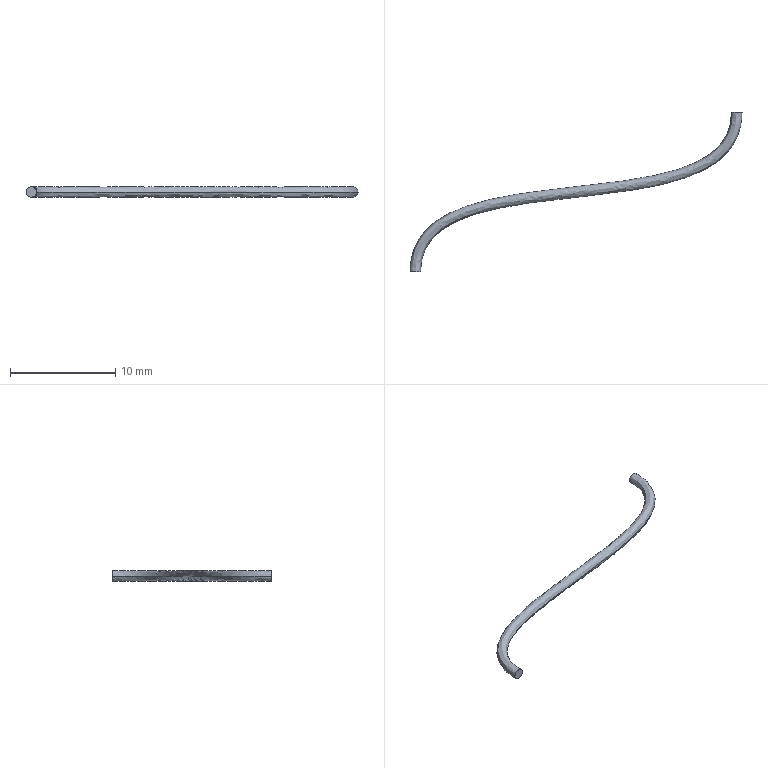Part | NX | features BREP 1 | 1 solid | 4 faces | box 31.607 x 15.16 x 1 mm | volume 29.37 mm3 | plane 2 | spline 2
STEP:
#1=CARTESIAN_POINT('',(-387.702,164.89,219.465));
#2=VERTEX_POINT('',#1);
#3=CARTESIAN_POINT('',(-388.702,164.89,219.465));
#4=VERTEX_POINT('',#3);
#5=CARTESIAN_POINT('',(-387.702,164.89,219.465));
#6=CARTESIAN_POINT('',(-387.702,164.89,219.524));
#7=CARTESIAN_POINT('',(-387.723,164.89,219.646));
#8=CARTESIAN_POINT('',(-387.827,164.89,219.815));
#9=CARTESIAN_POINT('',(-387.995,164.89,219.936));
#10=CARTESIAN_POINT('',(-388.202,164.89,219.98));
#11=CARTESIAN_POINT('',(-388.409,164.89,219.936));
#12=CARTESIAN_POINT('',(-388.577,164.89,219.815));
#13=CARTESIAN_POINT('',(-388.681,164.89,219.646));
#14=CARTESIAN_POINT('',(-388.702,164.89,219.524));
#15=CARTESIAN_POINT('',(-388.702,164.89,219.465));
#16=B_SPLINE_CURVE_WITH_KNOTS('',3,(#5,#6,#7,#8,#9,#10,#11,#12,#13,#14,#15),.UNSPECIFIED.,.F.,.F.,(4,1,1,1,1,1,1,1,4),(0.,0.125,0.25,0.375,0.5,0.625,0.75,0.875,1.),.UNSPECIFIED.);
#17=EDGE_CURVE('',#2,#4,#16,.T.);
#18=ORIENTED_EDGE('',*,*,#17,.F.);
#19=CARTESIAN_POINT('',(-388.702,164.89,219.465));
#20=CARTESIAN_POINT('',(-388.702,164.89,219.406));
#21=CARTESIAN_POINT('',(-388.681,164.89,219.284));
#22=CARTESIAN_POINT('',(-388.577,164.89,219.115));
#23=CARTESIAN_POINT('',(-388.409,164.89,218.994));
#24=CARTESIAN_POINT('',(-388.202,164.89,218.95));
#25=CARTESIAN_POINT('',(-387.995,164.89,218.994));
#26=CARTESIAN_POINT('',(-387.827,164.89,219.115));
#27=CARTESIAN_POINT('',(-387.723,164.89,219.284));
#28=CARTESIAN_POINT('',(-387.702,164.89,219.406));
#29=CARTESIAN_POINT('',(-387.702,164.89,219.465));
#30=B_SPLINE_CURVE_WITH_KNOTS('',3,(#19,#20,#21,#22,#23,#24,#25,#26,#27,#28,#29),.UNSPECIFIED.,.F.,.F.,(4,1,1,1,1,1,1,1,4),(0.,0.125,0.25,0.375,0.5,0.625,0.75,0.875,1.),.UNSPECIFIED.);
#31=EDGE_CURVE('',#4,#2,#30,.T.);
#32=ORIENTED_EDGE('',*,*,#31,.F.);
#33=EDGE_LOOP('',(#18,#32));
#34=FACE_BOUND('',#33,.T.);
#35=CARTESIAN_POINT('',(-387.702,164.89,219.465));
#36=DIRECTION('',(0.,1.,0.));
#37=DIRECTION('',(-1.,0.,0.));
#38=AXIS2_PLACEMENT_3D('',#35,#36,#37);
#39=PLANE('',#38);
#40=ADVANCED_FACE('',(#34),#39,.T.);
#41=CARTESIAN_POINT('',(-418.309,149.73,219.465));
#42=VERTEX_POINT('',#41);
#43=CARTESIAN_POINT('',(-418.309,149.73,219.465));
#44=CARTESIAN_POINT('',(-418.309,150.304,219.465));
#45=CARTESIAN_POINT('',(-418.189,151.148,219.465));
#46=CARTESIAN_POINT('',(-417.734,152.153,219.465));
#47=CARTESIAN_POINT('',(-417.005,153.18,219.465));
#48=CARTESIAN_POINT('',(-415.89,154.025,219.465));
#49=CARTESIAN_POINT('',(-414.532,154.685,219.465));
#50=CARTESIAN_POINT('',(-413.295,155.15,219.465));
#51=CARTESIAN_POINT('',(-411.827,155.564,219.465));
#52=CARTESIAN_POINT('',(-409.586,156.037,219.465));
#53=CARTESIAN_POINT('',(-406.748,156.447,219.465));
#54=CARTESIAN_POINT('',(-403.317,156.827,219.465));
#55=CARTESIAN_POINT('',(-399.918,157.208,219.465));
#56=CARTESIAN_POINT('',(-397.102,157.625,219.465));
#57=CARTESIAN_POINT('',(-394.881,158.102,219.465));
#58=CARTESIAN_POINT('',(-393.39,158.524,219.465));
#59=CARTESIAN_POINT('',(-392.088,159.012,219.465));
#60=CARTESIAN_POINT('',(-390.601,159.733,219.465));
#61=CARTESIAN_POINT('',(-389.301,160.706,219.465));
#62=CARTESIAN_POINT('',(-388.406,161.965,219.465));
#63=CARTESIAN_POINT('',(-387.844,163.208,219.465));
#64=CARTESIAN_POINT('',(-387.702,164.224,219.465));
#65=CARTESIAN_POINT('',(-387.702,164.89,219.465));
#66=B_SPLINE_CURVE_WITH_KNOTS('',3,(#43,#44,#45,#46,#47,#48,#49,#50,#51,#52,#53,#54,#55,#56,#57,#58,#59,#60,#61,#62,#63,#64,#65),.UNSPECIFIED.,.F.,.F.,(4,1,1,1,1,1,1,1,1,1,1,1,1,1,1,1,1,1,1,1,4),(0.,0.04977,0.07466,0.09954,0.1621,0.1934,0.2247,0.2715,0.3184,0.4121,0.5037,0.5953,0.6853,0.7303,0.7753,0.8066,0.8379,0.9005,0.9253,0.9502,1.),.UNSPECIFIED.);
#67=EDGE_CURVE('',#42,#2,#66,.T.);
#68=ORIENTED_EDGE('',*,*,#67,.T.);
#69=ORIENTED_EDGE('',*,*,#17,.T.);
#70=CARTESIAN_POINT('',(-419.309,149.73,219.465));
#71=VERTEX_POINT('',#70);
#72=CARTESIAN_POINT('',(-388.702,164.89,219.465));
#73=CARTESIAN_POINT('',(-388.702,164.316,219.465));
#74=CARTESIAN_POINT('',(-388.822,163.472,219.465));
#75=CARTESIAN_POINT('',(-389.277,162.467,219.465));
#76=CARTESIAN_POINT('',(-390.006,161.44,219.465));
#77=CARTESIAN_POINT('',(-391.121,160.595,219.465));
#78=CARTESIAN_POINT('',(-392.479,159.935,219.465));
#79=CARTESIAN_POINT('',(-393.696,159.477,219.465));
#80=CARTESIAN_POINT('',(-395.118,159.074,219.465));
#81=CARTESIAN_POINT('',(-397.271,158.611,219.465));
#82=CARTESIAN_POINT('',(-400.04,158.201,219.465));
#83=CARTESIAN_POINT('',(-403.423,157.822,219.465));
#84=CARTESIAN_POINT('',(-406.868,157.44,219.465));
#85=CARTESIAN_POINT('',(-409.751,157.024,219.465));
#86=CARTESIAN_POINT('',(-412.062,156.536,219.465));
#87=CARTESIAN_POINT('',(-413.599,156.104,219.465));
#88=CARTESIAN_POINT('',(-414.923,155.608,219.465));
#89=CARTESIAN_POINT('',(-416.41,154.887,219.465));
#90=CARTESIAN_POINT('',(-417.71,153.914,219.465));
#91=CARTESIAN_POINT('',(-418.605,152.655,219.465));
#92=CARTESIAN_POINT('',(-419.167,151.412,219.465));
#93=CARTESIAN_POINT('',(-419.309,150.396,219.465));
#94=CARTESIAN_POINT('',(-419.309,149.73,219.465));
#95=B_SPLINE_CURVE_WITH_KNOTS('',3,(#72,#73,#74,#75,#76,#77,#78,#79,#80,#81,#82,#83,#84,#85,#86,#87,#88,#89,#90,#91,#92,#93,#94),.UNSPECIFIED.,.F.,.F.,(4,1,1,1,1,1,1,1,1,1,1,1,1,1,1,1,1,1,1,1,4),(0.,0.04977,0.07466,0.09954,0.1621,0.1934,0.2247,0.2697,0.3147,0.4047,0.4963,0.5879,0.6816,0.7285,0.7753,0.8066,0.8379,0.9005,0.9253,0.9502,1.),.UNSPECIFIED.);
#96=EDGE_CURVE('',#4,#71,#95,.T.);
#97=ORIENTED_EDGE('',*,*,#96,.T.);
#98=CARTESIAN_POINT('',(-418.309,149.73,219.465));
#99=CARTESIAN_POINT('',(-418.309,149.73,219.524));
#100=CARTESIAN_POINT('',(-418.33,149.73,219.646));
#101=CARTESIAN_POINT('',(-418.434,149.73,219.815));
#102=CARTESIAN_POINT('',(-418.602,149.73,219.936));
#103=CARTESIAN_POINT('',(-418.809,149.73,219.98));
#104=CARTESIAN_POINT('',(-419.016,149.73,219.936));
#105=CARTESIAN_POINT('',(-419.184,149.73,219.815));
#106=CARTESIAN_POINT('',(-419.288,149.73,219.646));
#107=CARTESIAN_POINT('',(-419.309,149.73,219.524));
#108=CARTESIAN_POINT('',(-419.309,149.73,219.465));
#109=B_SPLINE_CURVE_WITH_KNOTS('',3,(#98,#99,#100,#101,#102,#103,#104,#105,#106,#107,#108),.UNSPECIFIED.,.F.,.F.,(4,1,1,1,1,1,1,1,4),(0.,0.125,0.25,0.375,0.5,0.625,0.75,0.875,1.),.UNSPECIFIED.);
#110=EDGE_CURVE('',#42,#71,#109,.T.);
#111=ORIENTED_EDGE('',*,*,#110,.F.);
#112=EDGE_LOOP('',(#68,#69,#97,#111));
#113=FACE_BOUND('',#112,.T.);
#114=CARTESIAN_POINT('',(-388.702,164.89,219.465));
#115=CARTESIAN_POINT('',(-388.702,164.89,219.524));
#116=CARTESIAN_POINT('',(-388.681,164.89,219.646));
#117=CARTESIAN_POINT('',(-388.577,164.89,219.815));
#118=CARTESIAN_POINT('',(-388.409,164.89,219.936));
#119=CARTESIAN_POINT('',(-388.202,164.89,219.98));
#120=CARTESIAN_POINT('',(-387.995,164.89,219.936));
#121=CARTESIAN_POINT('',(-387.827,164.89,219.815));
#122=CARTESIAN_POINT('',(-387.723,164.89,219.646));
#123=CARTESIAN_POINT('',(-387.702,164.89,219.524));
#124=CARTESIAN_POINT('',(-387.702,164.89,219.465));
#125=CARTESIAN_POINT('',(-388.702,164.316,219.465));
#126=CARTESIAN_POINT('',(-388.702,164.316,219.524));
#127=CARTESIAN_POINT('',(-388.681,164.314,219.646));
#128=CARTESIAN_POINT('',(-388.577,164.304,219.815));
#129=CARTESIAN_POINT('',(-388.409,164.289,219.936));
#130=CARTESIAN_POINT('',(-388.202,164.27,219.98));
#131=CARTESIAN_POINT('',(-387.995,164.251,219.936));
#132=CARTESIAN_POINT('',(-387.827,164.236,219.815));
#133=CARTESIAN_POINT('',(-387.723,164.226,219.646));
#134=CARTESIAN_POINT('',(-387.702,164.224,219.524));
#135=CARTESIAN_POINT('',(-387.702,164.224,219.465));
#136=CARTESIAN_POINT('',(-388.822,163.472,219.465));
#137=CARTESIAN_POINT('',(-388.822,163.472,219.524));
#138=CARTESIAN_POINT('',(-388.802,163.467,219.646));
#139=CARTESIAN_POINT('',(-388.7,163.439,219.815));
#140=CARTESIAN_POINT('',(-388.536,163.395,219.936));
#141=CARTESIAN_POINT('',(-388.333,163.34,219.98));
#142=CARTESIAN_POINT('',(-388.131,163.286,219.936));
#143=CARTESIAN_POINT('',(-387.966,163.241,219.815));
#144=CARTESIAN_POINT('',(-387.865,163.214,219.646));
#145=CARTESIAN_POINT('',(-387.844,163.208,219.524));
#146=CARTESIAN_POINT('',(-387.844,163.208,219.465));
#147=CARTESIAN_POINT('',(-389.277,162.467,219.465));
#148=CARTESIAN_POINT('',(-389.277,162.467,219.524));
#149=CARTESIAN_POINT('',(-389.259,162.457,219.646));
#150=CARTESIAN_POINT('',(-389.169,162.405,219.815));
#151=CARTESIAN_POINT('',(-389.022,162.32,219.936));
#152=CARTESIAN_POINT('',(-388.841,162.216,219.98));
#153=CARTESIAN_POINT('',(-388.661,162.112,219.936));
#154=CARTESIAN_POINT('',(-388.514,162.028,219.815));
#155=CARTESIAN_POINT('',(-388.424,161.976,219.646));
#156=CARTESIAN_POINT('',(-388.406,161.965,219.524));
#157=CARTESIAN_POINT('',(-388.406,161.965,219.465));
#158=CARTESIAN_POINT('',(-390.006,161.44,219.465));
#159=CARTESIAN_POINT('',(-390.006,161.44,219.524));
#160=CARTESIAN_POINT('',(-389.992,161.424,219.646));
#161=CARTESIAN_POINT('',(-389.918,161.348,219.815));
#162=CARTESIAN_POINT('',(-389.8,161.225,219.936));
#163=CARTESIAN_POINT('',(-389.654,161.073,219.98));
#164=CARTESIAN_POINT('',(-389.508,160.921,219.936));
#165=CARTESIAN_POINT('',(-389.389,160.798,219.815));
#166=CARTESIAN_POINT('',(-389.316,160.722,219.646));
#167=CARTESIAN_POINT('',(-389.301,160.706,219.524));
#168=CARTESIAN_POINT('',(-389.301,160.706,219.465));
#169=CARTESIAN_POINT('',(-391.121,160.595,219.465));
#170=CARTESIAN_POINT('',(-391.121,160.595,219.524));
#171=CARTESIAN_POINT('',(-391.11,160.577,219.646));
#172=CARTESIAN_POINT('',(-391.056,160.487,219.815));
#173=CARTESIAN_POINT('',(-390.969,160.342,219.936));
#174=CARTESIAN_POINT('',(-390.861,160.164,219.98));
#175=CARTESIAN_POINT('',(-390.753,159.985,219.936));
#176=CARTESIAN_POINT('',(-390.666,159.84,219.815));
#177=CARTESIAN_POINT('',(-390.612,159.751,219.646));
#178=CARTESIAN_POINT('',(-390.601,159.733,219.524));
#179=CARTESIAN_POINT('',(-390.601,159.733,219.465));
#180=CARTESIAN_POINT('',(-392.479,159.935,219.465));
#181=CARTESIAN_POINT('',(-392.479,159.935,219.524));
#182=CARTESIAN_POINT('',(-392.471,159.915,219.646));
#183=CARTESIAN_POINT('',(-392.43,159.82,219.815));
#184=CARTESIAN_POINT('',(-392.364,159.665,219.936));
#185=CARTESIAN_POINT('',(-392.283,159.474,219.98));
#186=CARTESIAN_POINT('',(-392.202,159.283,219.936));
#187=CARTESIAN_POINT('',(-392.137,159.127,219.815));
#188=CARTESIAN_POINT('',(-392.096,159.032,219.646));
#189=CARTESIAN_POINT('',(-392.088,159.012,219.524));
#190=CARTESIAN_POINT('',(-392.088,159.012,219.465));
#191=CARTESIAN_POINT('',(-393.696,159.477,219.465));
#192=CARTESIAN_POINT('',(-393.696,159.477,219.524));
#193=CARTESIAN_POINT('',(-393.689,159.457,219.646));
#194=CARTESIAN_POINT('',(-393.657,159.359,219.815));
#195=CARTESIAN_POINT('',(-393.606,159.198,219.936));
#196=CARTESIAN_POINT('',(-393.543,159.001,219.98));
#197=CARTESIAN_POINT('',(-393.479,158.803,219.936));
#198=CARTESIAN_POINT('',(-393.428,158.643,219.815));
#199=CARTESIAN_POINT('',(-393.396,158.544,219.646));
#200=CARTESIAN_POINT('',(-393.39,158.524,219.524));
#201=CARTESIAN_POINT('',(-393.39,158.524,219.465));
#202=CARTESIAN_POINT('',(-395.118,159.074,219.465));
#203=CARTESIAN_POINT('',(-395.118,159.074,219.524));
#204=CARTESIAN_POINT('',(-395.113,159.053,219.646));
#205=CARTESIAN_POINT('',(-395.089,158.952,219.815));
#206=CARTESIAN_POINT('',(-395.049,158.789,219.936));
#207=CARTESIAN_POINT('',(-395.,158.588,219.98));
#208=CARTESIAN_POINT('',(-394.95,158.386,219.936));
#209=CARTESIAN_POINT('',(-394.91,158.223,219.815));
#210=CARTESIAN_POINT('',(-394.886,158.122,219.646));
#211=CARTESIAN_POINT('',(-394.881,158.102,219.524));
#212=CARTESIAN_POINT('',(-394.881,158.102,219.465));
#213=CARTESIAN_POINT('',(-397.271,158.611,219.465));
#214=CARTESIAN_POINT('',(-397.271,158.611,219.524));
#215=CARTESIAN_POINT('',(-397.268,158.59,219.646));
#216=CARTESIAN_POINT('',(-397.25,158.488,219.815));
#217=CARTESIAN_POINT('',(-397.222,158.322,219.936));
#218=CARTESIAN_POINT('',(-397.187,158.118,219.98));
#219=CARTESIAN_POINT('',(-397.152,157.914,219.936));
#220=CARTESIAN_POINT('',(-397.123,157.748,219.815));
#221=CARTESIAN_POINT('',(-397.106,157.646,219.646));
#222=CARTESIAN_POINT('',(-397.102,157.625,219.524));
#223=CARTESIAN_POINT('',(-397.102,157.625,219.465));
#224=CARTESIAN_POINT('',(-400.04,158.201,219.465));
#225=CARTESIAN_POINT('',(-400.04,158.201,219.524));
#226=CARTESIAN_POINT('',(-400.038,158.18,219.646));
#227=CARTESIAN_POINT('',(-400.025,158.077,219.815));
#228=CARTESIAN_POINT('',(-400.004,157.91,219.936));
#229=CARTESIAN_POINT('',(-399.979,157.704,219.98));
#230=CARTESIAN_POINT('',(-399.954,157.499,219.936));
#231=CARTESIAN_POINT('',(-399.933,157.332,219.815));
#232=CARTESIAN_POINT('',(-399.92,157.229,219.646));
#233=CARTESIAN_POINT('',(-399.918,157.208,219.524));
#234=CARTESIAN_POINT('',(-399.918,157.208,219.465));
#235=CARTESIAN_POINT('',(-403.423,157.822,219.465));
#236=CARTESIAN_POINT('',(-403.423,157.822,219.524));
#237=CARTESIAN_POINT('',(-403.421,157.801,219.646));
#238=CARTESIAN_POINT('',(-403.41,157.698,219.815));
#239=CARTESIAN_POINT('',(-403.392,157.53,219.936));
#240=CARTESIAN_POINT('',(-403.37,157.324,219.98));
#241=CARTESIAN_POINT('',(-403.348,157.119,219.936));
#242=CARTESIAN_POINT('',(-403.331,156.951,219.815));
#243=CARTESIAN_POINT('',(-403.32,156.848,219.646));
#244=CARTESIAN_POINT('',(-403.317,156.827,219.524));
#245=CARTESIAN_POINT('',(-403.317,156.827,219.465));
#246=CARTESIAN_POINT('',(-406.868,157.44,219.465));
#247=CARTESIAN_POINT('',(-406.868,157.44,219.524));
#248=CARTESIAN_POINT('',(-406.866,157.419,219.646));
#249=CARTESIAN_POINT('',(-406.853,157.316,219.815));
#250=CARTESIAN_POINT('',(-406.833,157.149,219.936));
#251=CARTESIAN_POINT('',(-406.808,156.943,219.98));
#252=CARTESIAN_POINT('',(-406.783,156.738,219.936));
#253=CARTESIAN_POINT('',(-406.763,156.571,219.815));
#254=CARTESIAN_POINT('',(-406.75,156.468,219.646));
#255=CARTESIAN_POINT('',(-406.748,156.447,219.524));
#256=CARTESIAN_POINT('',(-406.748,156.447,219.465));
#257=CARTESIAN_POINT('',(-409.751,157.024,219.465));
#258=CARTESIAN_POINT('',(-409.751,157.024,219.524));
#259=CARTESIAN_POINT('',(-409.747,157.003,219.646));
#260=CARTESIAN_POINT('',(-409.73,156.901,219.815));
#261=CARTESIAN_POINT('',(-409.703,156.735,219.936));
#262=CARTESIAN_POINT('',(-409.668,156.531,219.98));
#263=CARTESIAN_POINT('',(-409.634,156.326,219.936));
#264=CARTESIAN_POINT('',(-409.606,156.16,219.815));
#265=CARTESIAN_POINT('',(-409.589,156.058,219.646));
#266=CARTESIAN_POINT('',(-409.586,156.037,219.524));
#267=CARTESIAN_POINT('',(-409.586,156.037,219.465));
#268=CARTESIAN_POINT('',(-412.062,156.536,219.465));
#269=CARTESIAN_POINT('',(-412.062,156.536,219.524));
#270=CARTESIAN_POINT('',(-412.057,156.516,219.646));
#271=CARTESIAN_POINT('',(-412.033,156.415,219.815));
#272=CARTESIAN_POINT('',(-411.993,156.251,219.936));
#273=CARTESIAN_POINT('',(-411.945,156.05,219.98));
#274=CARTESIAN_POINT('',(-411.896,155.849,219.936));
#275=CARTESIAN_POINT('',(-411.857,155.685,219.815));
#276=CARTESIAN_POINT('',(-411.832,155.584,219.646));
#277=CARTESIAN_POINT('',(-411.827,155.564,219.524));
#278=CARTESIAN_POINT('',(-411.827,155.564,219.465));
#279=CARTESIAN_POINT('',(-413.599,156.104,219.465));
#280=CARTESIAN_POINT('',(-413.599,156.104,219.524));
#281=CARTESIAN_POINT('',(-413.592,156.084,219.646));
#282=CARTESIAN_POINT('',(-413.561,155.985,219.815));
#283=CARTESIAN_POINT('',(-413.51,155.825,219.936));
#284=CARTESIAN_POINT('',(-413.447,155.627,219.98));
#285=CARTESIAN_POINT('',(-413.384,155.43,219.936));
#286=CARTESIAN_POINT('',(-413.333,155.269,219.815));
#287=CARTESIAN_POINT('',(-413.301,155.171,219.646));
#288=CARTESIAN_POINT('',(-413.295,155.15,219.524));
#289=CARTESIAN_POINT('',(-413.295,155.15,219.465));
#290=CARTESIAN_POINT('',(-414.923,155.608,219.465));
#291=CARTESIAN_POINT('',(-414.923,155.608,219.524));
#292=CARTESIAN_POINT('',(-414.915,155.588,219.646));
#293=CARTESIAN_POINT('',(-414.874,155.493,219.815));
#294=CARTESIAN_POINT('',(-414.809,155.337,219.936));
#295=CARTESIAN_POINT('',(-414.728,155.146,219.98));
#296=CARTESIAN_POINT('',(-414.647,154.955,219.936));
#297=CARTESIAN_POINT('',(-414.581,154.8,219.815));
#298=CARTESIAN_POINT('',(-414.54,154.705,219.646));
#299=CARTESIAN_POINT('',(-414.532,154.685,219.524));
#300=CARTESIAN_POINT('',(-414.532,154.685,219.465));
#301=CARTESIAN_POINT('',(-416.41,154.887,219.465));
#302=CARTESIAN_POINT('',(-416.41,154.887,219.524));
#303=CARTESIAN_POINT('',(-416.399,154.869,219.646));
#304=CARTESIAN_POINT('',(-416.345,154.78,219.815));
#305=CARTESIAN_POINT('',(-416.258,154.635,219.936));
#306=CARTESIAN_POINT('',(-416.15,154.456,219.98));
#307=CARTESIAN_POINT('',(-416.042,154.278,219.936));
#308=CARTESIAN_POINT('',(-415.955,154.133,219.815));
#309=CARTESIAN_POINT('',(-415.901,154.043,219.646));
#310=CARTESIAN_POINT('',(-415.89,154.025,219.524));
#311=CARTESIAN_POINT('',(-415.89,154.025,219.465));
#312=CARTESIAN_POINT('',(-417.71,153.914,219.465));
#313=CARTESIAN_POINT('',(-417.71,153.914,219.524));
#314=CARTESIAN_POINT('',(-417.695,153.898,219.646));
#315=CARTESIAN_POINT('',(-417.622,153.822,219.815));
#316=CARTESIAN_POINT('',(-417.503,153.699,219.936));
#317=CARTESIAN_POINT('',(-417.357,153.547,219.98));
#318=CARTESIAN_POINT('',(-417.211,153.395,219.936));
#319=CARTESIAN_POINT('',(-417.093,153.272,219.815));
#320=CARTESIAN_POINT('',(-417.019,153.196,219.646));
#321=CARTESIAN_POINT('',(-417.005,153.18,219.524));
#322=CARTESIAN_POINT('',(-417.005,153.18,219.465));
#323=CARTESIAN_POINT('',(-418.605,152.655,219.465));
#324=CARTESIAN_POINT('',(-418.605,152.655,219.524));
#325=CARTESIAN_POINT('',(-418.587,152.644,219.646));
#326=CARTESIAN_POINT('',(-418.497,152.592,219.815));
#327=CARTESIAN_POINT('',(-418.35,152.508,219.936));
#328=CARTESIAN_POINT('',(-418.17,152.404,219.98));
#329=CARTESIAN_POINT('',(-417.989,152.3,219.936));
#330=CARTESIAN_POINT('',(-417.842,152.215,219.815));
#331=CARTESIAN_POINT('',(-417.752,152.163,219.646));
#332=CARTESIAN_POINT('',(-417.734,152.153,219.524));
#333=CARTESIAN_POINT('',(-417.734,152.153,219.465));
#334=CARTESIAN_POINT('',(-419.167,151.412,219.465));
#335=CARTESIAN_POINT('',(-419.167,151.412,219.524));
#336=CARTESIAN_POINT('',(-419.146,151.406,219.646));
#337=CARTESIAN_POINT('',(-419.045,151.379,219.815));
#338=CARTESIAN_POINT('',(-418.88,151.334,219.936));
#339=CARTESIAN_POINT('',(-418.678,151.28,219.98));
#340=CARTESIAN_POINT('',(-418.475,151.225,219.936));
#341=CARTESIAN_POINT('',(-418.311,151.181,219.815));
#342=CARTESIAN_POINT('',(-418.209,151.153,219.646));
#343=CARTESIAN_POINT('',(-418.189,151.148,219.524));
#344=CARTESIAN_POINT('',(-418.189,151.148,219.465));
#345=CARTESIAN_POINT('',(-419.309,150.396,219.465));
#346=CARTESIAN_POINT('',(-419.309,150.396,219.524));
#347=CARTESIAN_POINT('',(-419.288,150.394,219.646));
#348=CARTESIAN_POINT('',(-419.184,150.384,219.815));
#349=CARTESIAN_POINT('',(-419.016,150.369,219.936));
#350=CARTESIAN_POINT('',(-418.809,150.35,219.98));
#351=CARTESIAN_POINT('',(-418.602,150.331,219.936));
#352=CARTESIAN_POINT('',(-418.434,150.316,219.815));
#353=CARTESIAN_POINT('',(-418.33,150.306,219.646));
#354=CARTESIAN_POINT('',(-418.309,150.304,219.524));
#355=CARTESIAN_POINT('',(-418.309,150.304,219.465));
#356=CARTESIAN_POINT('',(-419.309,149.73,219.465));
#357=CARTESIAN_POINT('',(-419.309,149.73,219.524));
#358=CARTESIAN_POINT('',(-419.288,149.73,219.646));
#359=CARTESIAN_POINT('',(-419.184,149.73,219.815));
#360=CARTESIAN_POINT('',(-419.016,149.73,219.936));
#361=CARTESIAN_POINT('',(-418.809,149.73,219.98));
#362=CARTESIAN_POINT('',(-418.602,149.73,219.936));
#363=CARTESIAN_POINT('',(-418.434,149.73,219.815));
#364=CARTESIAN_POINT('',(-418.33,149.73,219.646));
#365=CARTESIAN_POINT('',(-418.309,149.73,219.524));
#366=CARTESIAN_POINT('',(-418.309,149.73,219.465));
#367=B_SPLINE_SURFACE_WITH_KNOTS('',3,3,((#114,#115,#116,#117,#118,#119,#120,#121,#122,#123,#124),(#125,#126,#127,#128,#129,#130,#131,#132,#133,#134,#135),(#136,#137,#138,#139,#140,#141,#142,#143,#144,#145,#146),(#147,#148,#149,#150,#151,#152,#153,#154,#155,#156,#157),(#158,#159,#160,#161,#162,#163,#164,#165,#166,#167,#168),(#169,#170,#171,#172,#173,#174,#175,#176,#177,#178,#179),(#180,#181,#182,#183,#184,#185,#186,#187,#188,#189,#190),(#191,#192,#193,#194,#195,#196,#197,#198,#199,#200,#201),(#202,#203,#204,#205,#206,#207,#208,#209,#210,#211,#212),(#213,#214,#215,#216,#217,#218,#219,#220,#221,#222,#223),(#224,#225,#226,#227,#228,#229,#230,#231,#232,#233,#234),(#235,#236,#237,#238,#239,#240,#241,#242,#243,#244,#245),(#246,#247,#248,#249,#250,#251,#252,#253,#254,#255,#256),(#257,#258,#259,#260,#261,#262,#263,#264,#265,#266,#267),(#268,#269,#270,#271,#272,#273,#274,#275,#276,#277,#278),(#279,#280,#281,#282,#283,#284,#285,#286,#287,#288,#289),(#290,#291,#292,#293,#294,#295,#296,#297,#298,#299,#300),(#301,#302,#303,#304,#305,#306,#307,#308,#309,#310,#311),(#312,#313,#314,#315,#316,#317,#318,#319,#320,#321,#322),(#323,#324,#325,#326,#327,#328,#329,#330,#331,#332,#333),(#334,#335,#336,#337,#338,#339,#340,#341,#342,#343,#344),(#345,#346,#347,#348,#349,#350,#351,#352,#353,#354,#355),(#356,#357,#358,#359,#360,#361,#362,#363,#364,#365,#366)),.UNSPECIFIED.,.F.,.F.,.F.,(4,1,1,1,1,1,1,1,1,1,1,1,1,1,1,1,1,1,1,1,4),(4,1,1,1,1,1,1,1,4),(0.009182,0.05804,0.08247,0.1069,0.1683,0.199,0.2297,0.2739,0.3181,0.4065,0.4964,0.5863,0.6783,0.7243,0.7703,0.801,0.8317,0.8932,0.9176,0.942,0.9909),(0.01612,0.1371,0.2581,0.3791,0.5001,0.6211,0.7421,0.8631,0.984),.UNSPECIFIED.);
#368=ADVANCED_FACE('',(#113),#367,.T.);
#369=ORIENTED_EDGE('',*,*,#96,.F.);
#370=ORIENTED_EDGE('',*,*,#31,.T.);
#371=ORIENTED_EDGE('',*,*,#67,.F.);
#372=CARTESIAN_POINT('',(-419.309,149.73,219.465));
#373=CARTESIAN_POINT('',(-419.309,149.73,219.406));
#374=CARTESIAN_POINT('',(-419.288,149.73,219.284));
#375=CARTESIAN_POINT('',(-419.184,149.73,219.115));
#376=CARTESIAN_POINT('',(-419.016,149.73,218.994));
#377=CARTESIAN_POINT('',(-418.809,149.73,218.95));
#378=CARTESIAN_POINT('',(-418.602,149.73,218.994));
#379=CARTESIAN_POINT('',(-418.434,149.73,219.115));
#380=CARTESIAN_POINT('',(-418.33,149.73,219.284));
#381=CARTESIAN_POINT('',(-418.309,149.73,219.406));
#382=CARTESIAN_POINT('',(-418.309,149.73,219.465));
#383=B_SPLINE_CURVE_WITH_KNOTS('',3,(#372,#373,#374,#375,#376,#377,#378,#379,#380,#381,#382),.UNSPECIFIED.,.F.,.F.,(4,1,1,1,1,1,1,1,4),(0.,0.125,0.25,0.375,0.5,0.625,0.75,0.875,1.),.UNSPECIFIED.);
#384=EDGE_CURVE('',#71,#42,#383,.T.);
#385=ORIENTED_EDGE('',*,*,#384,.F.);
#386=EDGE_LOOP('',(#369,#370,#371,#385));
#387=FACE_BOUND('',#386,.T.);
#388=CARTESIAN_POINT('',(-387.702,164.89,219.465));
#389=CARTESIAN_POINT('',(-387.702,164.89,219.406));
#390=CARTESIAN_POINT('',(-387.723,164.89,219.284));
#391=CARTESIAN_POINT('',(-387.827,164.89,219.115));
#392=CARTESIAN_POINT('',(-387.995,164.89,218.994));
#393=CARTESIAN_POINT('',(-388.202,164.89,218.95));
#394=CARTESIAN_POINT('',(-388.409,164.89,218.994));
#395=CARTESIAN_POINT('',(-388.577,164.89,219.115));
#396=CARTESIAN_POINT('',(-388.681,164.89,219.284));
#397=CARTESIAN_POINT('',(-388.702,164.89,219.406));
#398=CARTESIAN_POINT('',(-388.702,164.89,219.465));
#399=CARTESIAN_POINT('',(-387.702,164.224,219.465));
#400=CARTESIAN_POINT('',(-387.702,164.224,219.406));
#401=CARTESIAN_POINT('',(-387.723,164.226,219.284));
#402=CARTESIAN_POINT('',(-387.827,164.236,219.115));
#403=CARTESIAN_POINT('',(-387.995,164.251,218.994));
#404=CARTESIAN_POINT('',(-388.202,164.27,218.95));
#405=CARTESIAN_POINT('',(-388.409,164.289,218.994));
#406=CARTESIAN_POINT('',(-388.577,164.304,219.115));
#407=CARTESIAN_POINT('',(-388.681,164.314,219.284));
#408=CARTESIAN_POINT('',(-388.702,164.316,219.406));
#409=CARTESIAN_POINT('',(-388.702,164.316,219.465));
#410=CARTESIAN_POINT('',(-387.844,163.208,219.465));
#411=CARTESIAN_POINT('',(-387.844,163.208,219.406));
#412=CARTESIAN_POINT('',(-387.865,163.214,219.284));
#413=CARTESIAN_POINT('',(-387.966,163.241,219.115));
#414=CARTESIAN_POINT('',(-388.131,163.286,218.994));
#415=CARTESIAN_POINT('',(-388.333,163.34,218.95));
#416=CARTESIAN_POINT('',(-388.536,163.395,218.994));
#417=CARTESIAN_POINT('',(-388.7,163.439,219.115));
#418=CARTESIAN_POINT('',(-388.802,163.467,219.284));
#419=CARTESIAN_POINT('',(-388.822,163.472,219.406));
#420=CARTESIAN_POINT('',(-388.822,163.472,219.465));
#421=CARTESIAN_POINT('',(-388.406,161.965,219.465));
#422=CARTESIAN_POINT('',(-388.406,161.965,219.406));
#423=CARTESIAN_POINT('',(-388.424,161.976,219.284));
#424=CARTESIAN_POINT('',(-388.514,162.028,219.115));
#425=CARTESIAN_POINT('',(-388.661,162.112,218.994));
#426=CARTESIAN_POINT('',(-388.841,162.216,218.95));
#427=CARTESIAN_POINT('',(-389.022,162.32,218.994));
#428=CARTESIAN_POINT('',(-389.169,162.405,219.115));
#429=CARTESIAN_POINT('',(-389.259,162.457,219.284));
#430=CARTESIAN_POINT('',(-389.277,162.467,219.406));
#431=CARTESIAN_POINT('',(-389.277,162.467,219.465));
#432=CARTESIAN_POINT('',(-389.301,160.706,219.465));
#433=CARTESIAN_POINT('',(-389.301,160.706,219.406));
#434=CARTESIAN_POINT('',(-389.316,160.722,219.284));
#435=CARTESIAN_POINT('',(-389.389,160.798,219.115));
#436=CARTESIAN_POINT('',(-389.508,160.921,218.994));
#437=CARTESIAN_POINT('',(-389.654,161.073,218.95));
#438=CARTESIAN_POINT('',(-389.8,161.225,218.994));
#439=CARTESIAN_POINT('',(-389.918,161.348,219.115));
#440=CARTESIAN_POINT('',(-389.992,161.424,219.284));
#441=CARTESIAN_POINT('',(-390.006,161.44,219.406));
#442=CARTESIAN_POINT('',(-390.006,161.44,219.465));
#443=CARTESIAN_POINT('',(-390.601,159.733,219.465));
#444=CARTESIAN_POINT('',(-390.601,159.733,219.406));
#445=CARTESIAN_POINT('',(-390.612,159.751,219.284));
#446=CARTESIAN_POINT('',(-390.666,159.84,219.115));
#447=CARTESIAN_POINT('',(-390.753,159.985,218.994));
#448=CARTESIAN_POINT('',(-390.861,160.164,218.95));
#449=CARTESIAN_POINT('',(-390.969,160.342,218.994));
#450=CARTESIAN_POINT('',(-391.056,160.487,219.115));
#451=CARTESIAN_POINT('',(-391.11,160.577,219.284));
#452=CARTESIAN_POINT('',(-391.121,160.595,219.406));
#453=CARTESIAN_POINT('',(-391.121,160.595,219.465));
#454=CARTESIAN_POINT('',(-392.088,159.012,219.465));
#455=CARTESIAN_POINT('',(-392.088,159.012,219.406));
#456=CARTESIAN_POINT('',(-392.096,159.032,219.284));
#457=CARTESIAN_POINT('',(-392.137,159.127,219.115));
#458=CARTESIAN_POINT('',(-392.202,159.283,218.994));
#459=CARTESIAN_POINT('',(-392.283,159.474,218.95));
#460=CARTESIAN_POINT('',(-392.364,159.665,218.994));
#461=CARTESIAN_POINT('',(-392.43,159.82,219.115));
#462=CARTESIAN_POINT('',(-392.471,159.915,219.284));
#463=CARTESIAN_POINT('',(-392.479,159.935,219.406));
#464=CARTESIAN_POINT('',(-392.479,159.935,219.465));
#465=CARTESIAN_POINT('',(-393.39,158.524,219.465));
#466=CARTESIAN_POINT('',(-393.39,158.524,219.406));
#467=CARTESIAN_POINT('',(-393.396,158.544,219.284));
#468=CARTESIAN_POINT('',(-393.428,158.643,219.115));
#469=CARTESIAN_POINT('',(-393.479,158.803,218.994));
#470=CARTESIAN_POINT('',(-393.543,159.001,218.95));
#471=CARTESIAN_POINT('',(-393.606,159.198,218.994));
#472=CARTESIAN_POINT('',(-393.657,159.359,219.115));
#473=CARTESIAN_POINT('',(-393.689,159.457,219.284));
#474=CARTESIAN_POINT('',(-393.696,159.477,219.406));
#475=CARTESIAN_POINT('',(-393.696,159.477,219.465));
#476=CARTESIAN_POINT('',(-394.881,158.102,219.465));
#477=CARTESIAN_POINT('',(-394.881,158.102,219.406));
#478=CARTESIAN_POINT('',(-394.886,158.122,219.284));
#479=CARTESIAN_POINT('',(-394.91,158.223,219.115));
#480=CARTESIAN_POINT('',(-394.95,158.386,218.994));
#481=CARTESIAN_POINT('',(-395.,158.588,218.95));
#482=CARTESIAN_POINT('',(-395.049,158.789,218.994));
#483=CARTESIAN_POINT('',(-395.089,158.952,219.115));
#484=CARTESIAN_POINT('',(-395.113,159.053,219.284));
#485=CARTESIAN_POINT('',(-395.118,159.074,219.406));
#486=CARTESIAN_POINT('',(-395.118,159.074,219.465));
#487=CARTESIAN_POINT('',(-397.102,157.625,219.465));
#488=CARTESIAN_POINT('',(-397.102,157.625,219.406));
#489=CARTESIAN_POINT('',(-397.106,157.646,219.284));
#490=CARTESIAN_POINT('',(-397.123,157.748,219.115));
#491=CARTESIAN_POINT('',(-397.152,157.914,218.994));
#492=CARTESIAN_POINT('',(-397.187,158.118,218.95));
#493=CARTESIAN_POINT('',(-397.222,158.322,218.994));
#494=CARTESIAN_POINT('',(-397.25,158.488,219.115));
#495=CARTESIAN_POINT('',(-397.268,158.59,219.284));
#496=CARTESIAN_POINT('',(-397.271,158.611,219.406));
#497=CARTESIAN_POINT('',(-397.271,158.611,219.465));
#498=CARTESIAN_POINT('',(-399.918,157.208,219.465));
#499=CARTESIAN_POINT('',(-399.918,157.208,219.406));
#500=CARTESIAN_POINT('',(-399.92,157.229,219.284));
#501=CARTESIAN_POINT('',(-399.933,157.332,219.115));
#502=CARTESIAN_POINT('',(-399.954,157.499,218.994));
#503=CARTESIAN_POINT('',(-399.979,157.704,218.95));
#504=CARTESIAN_POINT('',(-400.004,157.91,218.994));
#505=CARTESIAN_POINT('',(-400.025,158.077,219.115));
#506=CARTESIAN_POINT('',(-400.038,158.18,219.284));
#507=CARTESIAN_POINT('',(-400.04,158.201,219.406));
#508=CARTESIAN_POINT('',(-400.04,158.201,219.465));
#509=CARTESIAN_POINT('',(-403.317,156.827,219.465));
#510=CARTESIAN_POINT('',(-403.317,156.827,219.406));
#511=CARTESIAN_POINT('',(-403.32,156.848,219.284));
#512=CARTESIAN_POINT('',(-403.331,156.951,219.115));
#513=CARTESIAN_POINT('',(-403.348,157.119,218.994));
#514=CARTESIAN_POINT('',(-403.37,157.324,218.95));
#515=CARTESIAN_POINT('',(-403.392,157.53,218.994));
#516=CARTESIAN_POINT('',(-403.41,157.698,219.115));
#517=CARTESIAN_POINT('',(-403.421,157.801,219.284));
#518=CARTESIAN_POINT('',(-403.423,157.822,219.406));
#519=CARTESIAN_POINT('',(-403.423,157.822,219.465));
#520=CARTESIAN_POINT('',(-406.748,156.447,219.465));
#521=CARTESIAN_POINT('',(-406.748,156.447,219.406));
#522=CARTESIAN_POINT('',(-406.75,156.468,219.284));
#523=CARTESIAN_POINT('',(-406.763,156.571,219.115));
#524=CARTESIAN_POINT('',(-406.783,156.738,218.994));
#525=CARTESIAN_POINT('',(-406.808,156.943,218.95));
#526=CARTESIAN_POINT('',(-406.833,157.149,218.994));
#527=CARTESIAN_POINT('',(-406.853,157.316,219.115));
#528=CARTESIAN_POINT('',(-406.866,157.419,219.284));
#529=CARTESIAN_POINT('',(-406.868,157.44,219.406));
#530=CARTESIAN_POINT('',(-406.868,157.44,219.465));
#531=CARTESIAN_POINT('',(-409.586,156.037,219.465));
#532=CARTESIAN_POINT('',(-409.586,156.037,219.406));
#533=CARTESIAN_POINT('',(-409.589,156.058,219.284));
#534=CARTESIAN_POINT('',(-409.606,156.16,219.115));
#535=CARTESIAN_POINT('',(-409.634,156.326,218.994));
#536=CARTESIAN_POINT('',(-409.668,156.531,218.95));
#537=CARTESIAN_POINT('',(-409.703,156.735,218.994));
#538=CARTESIAN_POINT('',(-409.73,156.901,219.115));
#539=CARTESIAN_POINT('',(-409.747,157.003,219.284));
#540=CARTESIAN_POINT('',(-409.751,157.024,219.406));
#541=CARTESIAN_POINT('',(-409.751,157.024,219.465));
#542=CARTESIAN_POINT('',(-411.827,155.564,219.465));
#543=CARTESIAN_POINT('',(-411.827,155.564,219.406));
#544=CARTESIAN_POINT('',(-411.832,155.584,219.284));
#545=CARTESIAN_POINT('',(-411.857,155.685,219.115));
#546=CARTESIAN_POINT('',(-411.896,155.849,218.994));
#547=CARTESIAN_POINT('',(-411.945,156.05,218.95));
#548=CARTESIAN_POINT('',(-411.993,156.251,218.994));
#549=CARTESIAN_POINT('',(-412.033,156.415,219.115));
#550=CARTESIAN_POINT('',(-412.057,156.516,219.284));
#551=CARTESIAN_POINT('',(-412.062,156.536,219.406));
#552=CARTESIAN_POINT('',(-412.062,156.536,219.465));
#553=CARTESIAN_POINT('',(-413.295,155.15,219.465));
#554=CARTESIAN_POINT('',(-413.295,155.15,219.406));
#555=CARTESIAN_POINT('',(-413.301,155.171,219.284));
#556=CARTESIAN_POINT('',(-413.333,155.269,219.115));
#557=CARTESIAN_POINT('',(-413.384,155.43,218.994));
#558=CARTESIAN_POINT('',(-413.447,155.627,218.95));
#559=CARTESIAN_POINT('',(-413.51,155.825,218.994));
#560=CARTESIAN_POINT('',(-413.561,155.985,219.115));
#561=CARTESIAN_POINT('',(-413.592,156.084,219.284));
#562=CARTESIAN_POINT('',(-413.599,156.104,219.406));
#563=CARTESIAN_POINT('',(-413.599,156.104,219.465));
#564=CARTESIAN_POINT('',(-414.532,154.685,219.465));
#565=CARTESIAN_POINT('',(-414.532,154.685,219.406));
#566=CARTESIAN_POINT('',(-414.54,154.705,219.284));
#567=CARTESIAN_POINT('',(-414.581,154.8,219.115));
#568=CARTESIAN_POINT('',(-414.647,154.955,218.994));
#569=CARTESIAN_POINT('',(-414.728,155.146,218.95));
#570=CARTESIAN_POINT('',(-414.809,155.337,218.994));
#571=CARTESIAN_POINT('',(-414.874,155.493,219.115));
#572=CARTESIAN_POINT('',(-414.915,155.588,219.284));
#573=CARTESIAN_POINT('',(-414.923,155.608,219.406));
#574=CARTESIAN_POINT('',(-414.923,155.608,219.465));
#575=CARTESIAN_POINT('',(-415.89,154.025,219.465));
#576=CARTESIAN_POINT('',(-415.89,154.025,219.406));
#577=CARTESIAN_POINT('',(-415.901,154.043,219.284));
#578=CARTESIAN_POINT('',(-415.955,154.133,219.115));
#579=CARTESIAN_POINT('',(-416.042,154.278,218.994));
#580=CARTESIAN_POINT('',(-416.15,154.456,218.95));
#581=CARTESIAN_POINT('',(-416.258,154.635,218.994));
#582=CARTESIAN_POINT('',(-416.345,154.78,219.115));
#583=CARTESIAN_POINT('',(-416.399,154.869,219.284));
#584=CARTESIAN_POINT('',(-416.41,154.887,219.406));
#585=CARTESIAN_POINT('',(-416.41,154.887,219.465));
#586=CARTESIAN_POINT('',(-417.005,153.18,219.465));
#587=CARTESIAN_POINT('',(-417.005,153.18,219.406));
#588=CARTESIAN_POINT('',(-417.019,153.196,219.284));
#589=CARTESIAN_POINT('',(-417.093,153.272,219.115));
#590=CARTESIAN_POINT('',(-417.211,153.395,218.994));
#591=CARTESIAN_POINT('',(-417.357,153.547,218.95));
#592=CARTESIAN_POINT('',(-417.503,153.699,218.994));
#593=CARTESIAN_POINT('',(-417.622,153.822,219.115));
#594=CARTESIAN_POINT('',(-417.695,153.898,219.284));
#595=CARTESIAN_POINT('',(-417.71,153.914,219.406));
#596=CARTESIAN_POINT('',(-417.71,153.914,219.465));
#597=CARTESIAN_POINT('',(-417.734,152.153,219.465));
#598=CARTESIAN_POINT('',(-417.734,152.153,219.406));
#599=CARTESIAN_POINT('',(-417.752,152.163,219.284));
#600=CARTESIAN_POINT('',(-417.842,152.215,219.115));
#601=CARTESIAN_POINT('',(-417.989,152.3,218.994));
#602=CARTESIAN_POINT('',(-418.17,152.404,218.95));
#603=CARTESIAN_POINT('',(-418.35,152.508,218.994));
#604=CARTESIAN_POINT('',(-418.497,152.592,219.115));
#605=CARTESIAN_POINT('',(-418.587,152.644,219.284));
#606=CARTESIAN_POINT('',(-418.605,152.655,219.406));
#607=CARTESIAN_POINT('',(-418.605,152.655,219.465));
#608=CARTESIAN_POINT('',(-418.189,151.148,219.465));
#609=CARTESIAN_POINT('',(-418.189,151.148,219.406));
#610=CARTESIAN_POINT('',(-418.209,151.153,219.284));
#611=CARTESIAN_POINT('',(-418.311,151.181,219.115));
#612=CARTESIAN_POINT('',(-418.475,151.225,218.994));
#613=CARTESIAN_POINT('',(-418.678,151.28,218.95));
#614=CARTESIAN_POINT('',(-418.88,151.334,218.994));
#615=CARTESIAN_POINT('',(-419.045,151.379,219.115));
#616=CARTESIAN_POINT('',(-419.146,151.406,219.284));
#617=CARTESIAN_POINT('',(-419.167,151.412,219.406));
#618=CARTESIAN_POINT('',(-419.167,151.412,219.465));
#619=CARTESIAN_POINT('',(-418.309,150.304,219.465));
#620=CARTESIAN_POINT('',(-418.309,150.304,219.406));
#621=CARTESIAN_POINT('',(-418.33,150.306,219.284));
#622=CARTESIAN_POINT('',(-418.434,150.316,219.115));
#623=CARTESIAN_POINT('',(-418.602,150.331,218.994));
#624=CARTESIAN_POINT('',(-418.809,150.35,218.95));
#625=CARTESIAN_POINT('',(-419.016,150.369,218.994));
#626=CARTESIAN_POINT('',(-419.184,150.384,219.115));
#627=CARTESIAN_POINT('',(-419.288,150.394,219.284));
#628=CARTESIAN_POINT('',(-419.309,150.396,219.406));
#629=CARTESIAN_POINT('',(-419.309,150.396,219.465));
#630=CARTESIAN_POINT('',(-418.309,149.73,219.465));
#631=CARTESIAN_POINT('',(-418.309,149.73,219.406));
#632=CARTESIAN_POINT('',(-418.33,149.73,219.284));
#633=CARTESIAN_POINT('',(-418.434,149.73,219.115));
#634=CARTESIAN_POINT('',(-418.602,149.73,218.994));
#635=CARTESIAN_POINT('',(-418.809,149.73,218.95));
#636=CARTESIAN_POINT('',(-419.016,149.73,218.994));
#637=CARTESIAN_POINT('',(-419.184,149.73,219.115));
#638=CARTESIAN_POINT('',(-419.288,149.73,219.284));
#639=CARTESIAN_POINT('',(-419.309,149.73,219.406));
#640=CARTESIAN_POINT('',(-419.309,149.73,219.465));
#641=B_SPLINE_SURFACE_WITH_KNOTS('',3,3,((#388,#389,#390,#391,#392,#393,#394,#395,#396,#397,#398),(#399,#400,#401,#402,#403,#404,#405,#406,#407,#408,#409),(#410,#411,#412,#413,#414,#415,#416,#417,#418,#419,#420),(#421,#422,#423,#424,#425,#426,#427,#428,#429,#430,#431),(#432,#433,#434,#435,#436,#437,#438,#439,#440,#441,#442),(#443,#444,#445,#446,#447,#448,#449,#450,#451,#452,#453),(#454,#455,#456,#457,#458,#459,#460,#461,#462,#463,#464),(#465,#466,#467,#468,#469,#470,#471,#472,#473,#474,#475),(#476,#477,#478,#479,#480,#481,#482,#483,#484,#485,#486),(#487,#488,#489,#490,#491,#492,#493,#494,#495,#496,#497),(#498,#499,#500,#501,#502,#503,#504,#505,#506,#507,#508),(#509,#510,#511,#512,#513,#514,#515,#516,#517,#518,#519),(#520,#521,#522,#523,#524,#525,#526,#527,#528,#529,#530),(#531,#532,#533,#534,#535,#536,#537,#538,#539,#540,#541),(#542,#543,#544,#545,#546,#547,#548,#549,#550,#551,#552),(#553,#554,#555,#556,#557,#558,#559,#560,#561,#562,#563),(#564,#565,#566,#567,#568,#569,#570,#571,#572,#573,#574),(#575,#576,#577,#578,#579,#580,#581,#582,#583,#584,#585),(#586,#587,#588,#589,#590,#591,#592,#593,#594,#595,#596),(#597,#598,#599,#600,#601,#602,#603,#604,#605,#606,#607),(#608,#609,#610,#611,#612,#613,#614,#615,#616,#617,#618),(#619,#620,#621,#622,#623,#624,#625,#626,#627,#628,#629),(#630,#631,#632,#633,#634,#635,#636,#637,#638,#639,#640)),.UNSPECIFIED.,.F.,.F.,.F.,(4,1,1,1,1,1,1,1,1,1,1,1,1,1,1,1,1,1,1,1,4),(4,1,1,1,1,1,1,1,4),(0.009182,0.05804,0.08247,0.1069,0.1683,0.199,0.2297,0.2739,0.3181,0.4065,0.4964,0.5863,0.6783,0.7243,0.7703,0.801,0.8317,0.8932,0.9176,0.942,0.9909),(0.01612,0.1371,0.2581,0.3791,0.5001,0.6211,0.7421,0.8631,0.984),.UNSPECIFIED.);
#642=ADVANCED_FACE('',(#387),#641,.T.);
#643=ORIENTED_EDGE('',*,*,#384,.T.);
#644=ORIENTED_EDGE('',*,*,#110,.T.);
#645=EDGE_LOOP('',(#643,#644));
#646=FACE_BOUND('',#645,.T.);
#647=CARTESIAN_POINT('',(-418.309,149.73,219.465));
#648=DIRECTION('',(0.,1.,0.));
#649=DIRECTION('',(-1.,0.,0.));
#650=AXIS2_PLACEMENT_3D('',#647,#648,#649);
#651=PLANE('',#650);
#652=ADVANCED_FACE('',(#646),#651,.F.);
#653=CLOSED_SHELL('',(#40,#368,#642,#652));
#654=MANIFOLD_SOLID_BREP('',#653);
#655=(LENGTH_UNIT()NAMED_UNIT(*)SI_UNIT(.MILLI.,.METRE.));
#656=UNCERTAINTY_MEASURE_WITH_UNIT(LENGTH_MEASURE(0.00001),#655,'','');
#657=(NAMED_UNIT(*)PLANE_ANGLE_UNIT()SI_UNIT($,.RADIAN.));
#658=(NAMED_UNIT(*)SI_UNIT($,.STERADIAN.)SOLID_ANGLE_UNIT());
#659=(GEOMETRIC_REPRESENTATION_CONTEXT(3)GLOBAL_UNCERTAINTY_ASSIGNED_CONTEXT((#656))GLOBAL_UNIT_ASSIGNED_CONTEXT((#655,#657,#658))REPRESENTATION_CONTEXT('',''));
#660=ADVANCED_BREP_SHAPE_REPRESENTATION('',(#654),#659);